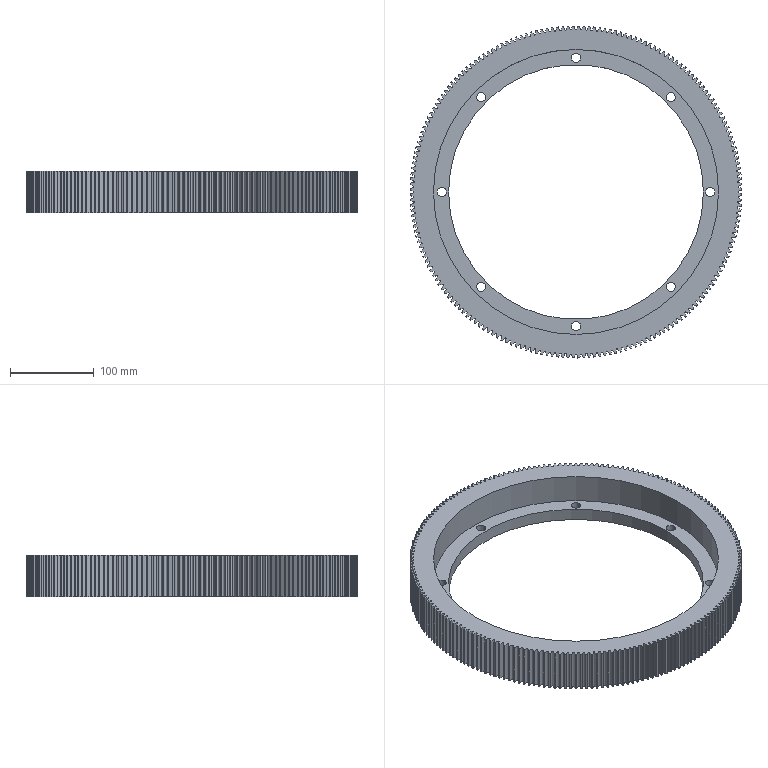Part | SolidWorks | features ICE 3, CirPattern 1, RefAxis 1, RevCut 1, Revolution 1 | 1 solid | 415 faces | box 395.972 x 395.972 x 50 mm | volume 1324995 mm3 | cylinder 216 | spline 196 | plane 3 | commonest cylinder face diameters 396 x196 11 x16 304 x2 340 x2